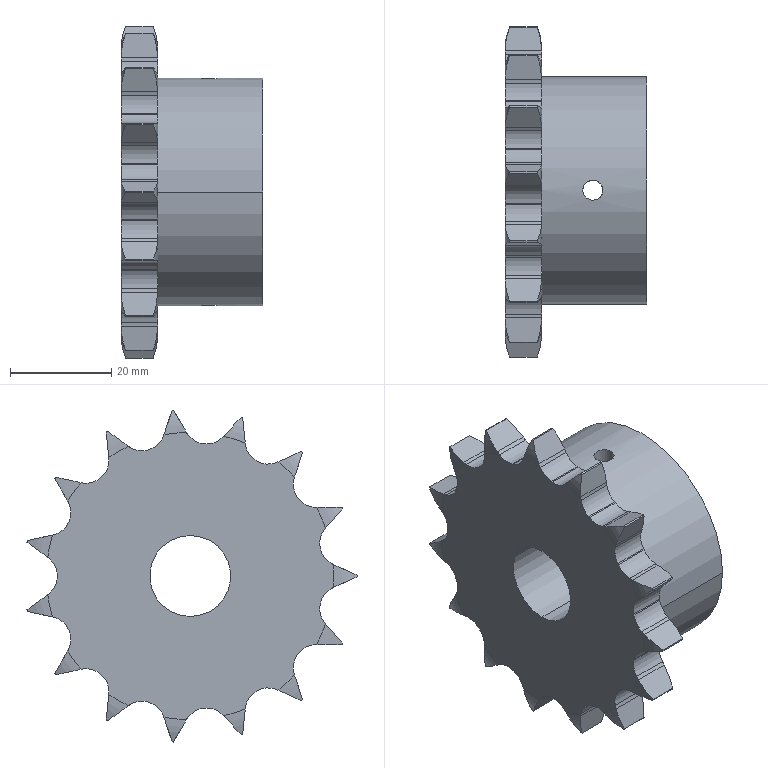Part | STEP file | 2108-151V11 | 1 solid | 161 faces | box 28 x 65.312 x 65.671 mm | volume 45287 mm3 | cylinder 83 | plane 48 | torus 30 | commonest cylinder face diameters 8.561 x30 22.126 x30 66 x15 4 x4 16 x2 45 x2